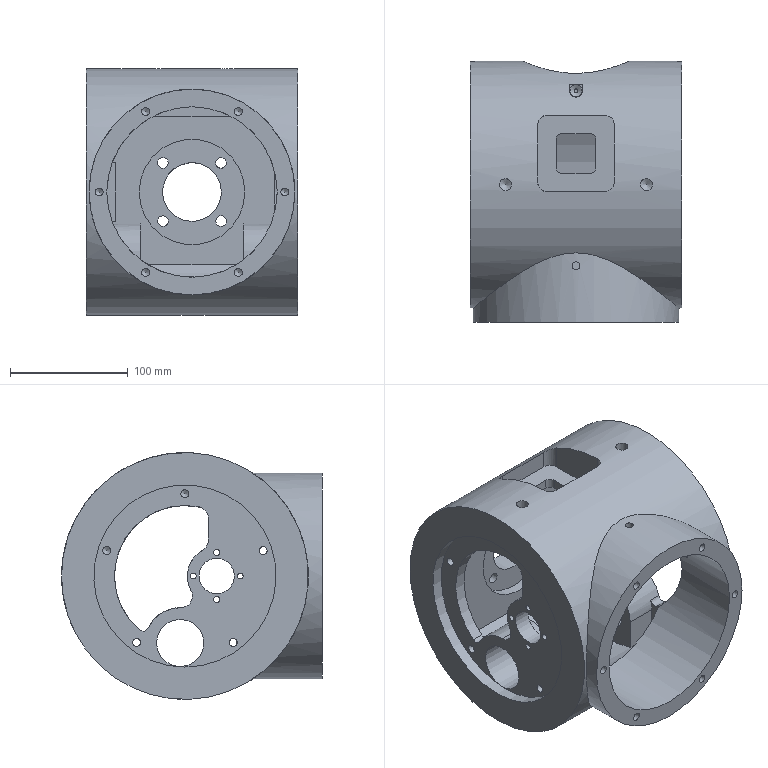Part | NX | features SYMBOLIC_THREAD 23, DATUM_CSYS 18, SKETCH 17, IDENTICAL INSTANCE OUTPUT 16, SIMPLE HOLE 16, EXTRUDE 15, Instance Feature 13, HOLE PACKAGE 12, MASTER SNAPSHOT BODY 4, Pattern Feature 3, BLEND 2, DATUM_PLANE 2, EXTRACT_STRING 2, CBORE_HOLE 1, DELETE FACE 1, Mirror Feature 1, SUBTRACT 1 | 1 solid | 125 faces | box 180 x 222 x 210 mm | volume 2622757 mm3 | cylinder 66 | plane 44 | cone 15 | commonest cylinder face diameters 6.8 x17 10 x8 5 x5 9 x4 14 x4 16 x4